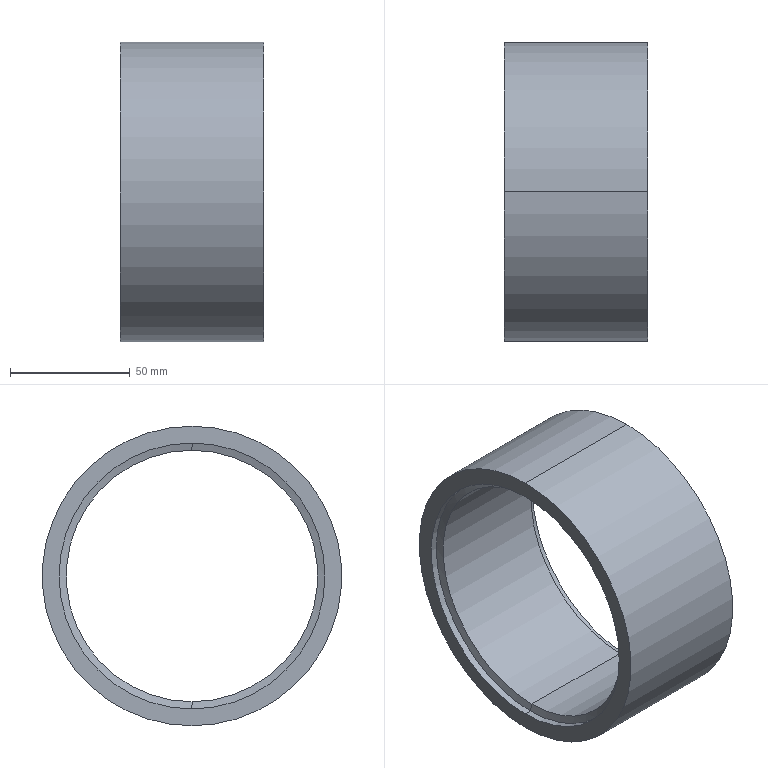Part | SolidWorks | features BaseBody 1 | 1 solid | 14 faces | box 60 x 125 x 125 mm | volume 209654 mm3 | cylinder 8 | cone 4 | plane 2 | commonest cylinder face diameters 111 x4 105 x2 125 x2
STEP:
#1=CARTESIAN_POINT('',(-30.,0.,-62.5));
#2=VERTEX_POINT('',#1);
#3=CARTESIAN_POINT('',(-30.,0.,62.5));
#4=VERTEX_POINT('',#3);
#5=CARTESIAN_POINT('',(-30.,0.,0.));
#6=DIRECTION('',(1.,0.,0.));
#7=DIRECTION('',(0.,0.,-1.));
#8=AXIS2_PLACEMENT_3D('',#5,#6,#7);
#9=CIRCLE('',#8,62.5);
#10=EDGE_CURVE('',#2,#4,#9,.T.);
#11=ORIENTED_EDGE('',*,*,#10,.T.);
#12=CARTESIAN_POINT('',(30.,0.,62.5));
#13=VERTEX_POINT('',#12);
#14=CARTESIAN_POINT('',(-33.,0.,62.5));
#15=DIRECTION('',(1.,0.,0.));
#16=VECTOR('',#15,1000.);
#17=LINE('',#14,#16);
#18=EDGE_CURVE('',#4,#13,#17,.T.);
#19=ORIENTED_EDGE('',*,*,#18,.T.);
#20=CARTESIAN_POINT('',(30.,0.,-62.5));
#21=VERTEX_POINT('',#20);
#22=CARTESIAN_POINT('',(30.,0.,0.));
#23=DIRECTION('',(-1.,0.,0.));
#24=DIRECTION('',(0.,0.,-1.));
#25=AXIS2_PLACEMENT_3D('',#22,#23,#24);
#26=CIRCLE('',#25,62.5);
#27=EDGE_CURVE('',#13,#21,#26,.T.);
#28=ORIENTED_EDGE('',*,*,#27,.T.);
#29=CARTESIAN_POINT('',(-33.,0.,-62.5));
#30=DIRECTION('',(1.,0.,0.));
#31=VECTOR('',#30,1000.);
#32=LINE('',#29,#31);
#33=EDGE_CURVE('',#2,#21,#32,.T.);
#34=ORIENTED_EDGE('',*,*,#33,.F.);
#35=EDGE_LOOP('',(#11,#19,#28,#34));
#36=FACE_OUTER_BOUND('',#35,.T.);
#37=CARTESIAN_POINT('',(-33.,0.,0.));
#38=DIRECTION('',(1.,0.,0.));
#39=DIRECTION('',(0.,0.,-1.));
#40=AXIS2_PLACEMENT_3D('',#37,#38,#39);
#41=CYLINDRICAL_SURFACE('',#40,62.5);
#42=ADVANCED_FACE('',(#36),#41,.T.);
#43=CARTESIAN_POINT('',(27.,0.,55.5));
#44=VERTEX_POINT('',#43);
#45=CARTESIAN_POINT('',(27.,0.,-55.5));
#46=VERTEX_POINT('',#45);
#47=CARTESIAN_POINT('',(27.,0.,0.));
#48=DIRECTION('',(1.,0.,0.));
#49=DIRECTION('',(0.,0.,-1.));
#50=AXIS2_PLACEMENT_3D('',#47,#48,#49);
#51=CIRCLE('',#50,55.5);
#52=EDGE_CURVE('',#44,#46,#51,.T.);
#53=ORIENTED_EDGE('',*,*,#52,.F.);
#54=CARTESIAN_POINT('',(30.,0.,55.5));
#55=VERTEX_POINT('',#54);
#56=CARTESIAN_POINT('',(-33.,0.,55.5));
#57=DIRECTION('',(1.,0.,0.));
#58=VECTOR('',#57,1000.);
#59=LINE('',#56,#58);
#60=EDGE_CURVE('',#44,#55,#59,.T.);
#61=ORIENTED_EDGE('',*,*,#60,.T.);
#62=CARTESIAN_POINT('',(30.,0.,-55.5));
#63=VERTEX_POINT('',#62);
#64=CARTESIAN_POINT('',(30.,0.,0.));
#65=DIRECTION('',(-1.,0.,0.));
#66=DIRECTION('',(0.,0.,-1.));
#67=AXIS2_PLACEMENT_3D('',#64,#65,#66);
#68=CIRCLE('',#67,55.5);
#69=EDGE_CURVE('',#63,#55,#68,.T.);
#70=ORIENTED_EDGE('',*,*,#69,.F.);
#71=CARTESIAN_POINT('',(-33.,0.,-55.5));
#72=DIRECTION('',(1.,0.,0.));
#73=VECTOR('',#72,1000.);
#74=LINE('',#71,#73);
#75=EDGE_CURVE('',#46,#63,#74,.T.);
#76=ORIENTED_EDGE('',*,*,#75,.F.);
#77=EDGE_LOOP('',(#53,#61,#70,#76));
#78=FACE_OUTER_BOUND('',#77,.T.);
#79=CARTESIAN_POINT('',(-33.,0.,0.));
#80=DIRECTION('',(1.,0.,0.));
#81=DIRECTION('',(0.,0.,-1.));
#82=AXIS2_PLACEMENT_3D('',#79,#80,#81);
#83=CYLINDRICAL_SURFACE('',#82,55.5);
#84=ADVANCED_FACE('',(#78),#83,.F.);
#85=CARTESIAN_POINT('',(-30.,0.,-55.5));
#86=VERTEX_POINT('',#85);
#87=CARTESIAN_POINT('',(-30.,0.,55.5));
#88=VERTEX_POINT('',#87);
#89=CARTESIAN_POINT('',(-30.,0.,0.));
#90=DIRECTION('',(-1.,0.,0.));
#91=DIRECTION('',(0.,0.,-1.));
#92=AXIS2_PLACEMENT_3D('',#89,#90,#91);
#93=CIRCLE('',#92,55.5);
#94=EDGE_CURVE('',#86,#88,#93,.T.);
#95=ORIENTED_EDGE('',*,*,#94,.T.);
#96=CARTESIAN_POINT('',(-27.,0.,55.5));
#97=VERTEX_POINT('',#96);
#98=CARTESIAN_POINT('',(-33.,0.,55.5));
#99=DIRECTION('',(1.,0.,0.));
#100=VECTOR('',#99,1000.);
#101=LINE('',#98,#100);
#102=EDGE_CURVE('',#88,#97,#101,.T.);
#103=ORIENTED_EDGE('',*,*,#102,.T.);
#104=CARTESIAN_POINT('',(-27.,0.,-55.5));
#105=VERTEX_POINT('',#104);
#106=CARTESIAN_POINT('',(-27.,0.,0.));
#107=DIRECTION('',(-1.,0.,0.));
#108=DIRECTION('',(0.,0.,-1.));
#109=AXIS2_PLACEMENT_3D('',#106,#107,#108);
#110=CIRCLE('',#109,55.5);
#111=EDGE_CURVE('',#105,#97,#110,.T.);
#112=ORIENTED_EDGE('',*,*,#111,.F.);
#113=CARTESIAN_POINT('',(-33.,0.,-55.5));
#114=DIRECTION('',(1.,0.,0.));
#115=VECTOR('',#114,1000.);
#116=LINE('',#113,#115);
#117=EDGE_CURVE('',#86,#105,#116,.T.);
#118=ORIENTED_EDGE('',*,*,#117,.F.);
#119=EDGE_LOOP('',(#95,#103,#112,#118));
#120=FACE_OUTER_BOUND('',#119,.T.);
#121=CARTESIAN_POINT('',(-33.,0.,0.));
#122=DIRECTION('',(1.,0.,0.));
#123=DIRECTION('',(0.,0.,-1.));
#124=AXIS2_PLACEMENT_3D('',#121,#122,#123);
#125=CYLINDRICAL_SURFACE('',#124,55.5);
#126=ADVANCED_FACE('',(#120),#125,.F.);
#127=CARTESIAN_POINT('',(26.,0.,52.5));
#128=VERTEX_POINT('',#127);
#129=CARTESIAN_POINT('',(26.,0.,-52.5));
#130=VERTEX_POINT('',#129);
#131=CARTESIAN_POINT('',(26.,0.,0.));
#132=DIRECTION('',(1.,0.,0.));
#133=DIRECTION('',(0.,0.,1.));
#134=AXIS2_PLACEMENT_3D('',#131,#132,#133);
#135=CIRCLE('',#134,52.5);
#136=EDGE_CURVE('',#128,#130,#135,.T.);
#137=ORIENTED_EDGE('',*,*,#136,.F.);
#138=CARTESIAN_POINT('',(27.,0.,55.5));
#139=DIRECTION('',(0.3162,0.,0.9487));
#140=VECTOR('',#139,1000.);
#141=LINE('',#138,#140);
#142=EDGE_CURVE('',#128,#44,#141,.T.);
#143=ORIENTED_EDGE('',*,*,#142,.T.);
#144=ORIENTED_EDGE('',*,*,#52,.T.);
#145=CARTESIAN_POINT('',(27.,0.,-55.5));
#146=DIRECTION('',(0.3162,0.,-0.9487));
#147=VECTOR('',#146,1000.);
#148=LINE('',#145,#147);
#149=EDGE_CURVE('',#130,#46,#148,.T.);
#150=ORIENTED_EDGE('',*,*,#149,.F.);
#151=EDGE_LOOP('',(#137,#143,#144,#150));
#152=FACE_OUTER_BOUND('',#151,.T.);
#153=CARTESIAN_POINT('',(27.,0.,0.));
#154=DIRECTION('',(1.,0.,0.));
#155=DIRECTION('',(0.,0.,-1.));
#156=AXIS2_PLACEMENT_3D('',#153,#154,#155);
#157=CONICAL_SURFACE('',#156,55.5,1.249);
#158=ADVANCED_FACE('',(#152),#157,.F.);
#159=CARTESIAN_POINT('',(-26.,0.,-52.5));
#160=VERTEX_POINT('',#159);
#161=CARTESIAN_POINT('',(-26.,0.,52.5));
#162=VERTEX_POINT('',#161);
#163=CARTESIAN_POINT('',(-26.,0.,0.));
#164=DIRECTION('',(-1.,0.,0.));
#165=DIRECTION('',(0.,0.,-1.));
#166=AXIS2_PLACEMENT_3D('',#163,#164,#165);
#167=CIRCLE('',#166,52.5);
#168=EDGE_CURVE('',#160,#162,#167,.T.);
#169=ORIENTED_EDGE('',*,*,#168,.F.);
#170=CARTESIAN_POINT('',(-27.,0.,-55.5));
#171=DIRECTION('',(-0.3162,0.,-0.9487));
#172=VECTOR('',#171,1000.);
#173=LINE('',#170,#172);
#174=EDGE_CURVE('',#160,#105,#173,.T.);
#175=ORIENTED_EDGE('',*,*,#174,.T.);
#176=ORIENTED_EDGE('',*,*,#111,.T.);
#177=CARTESIAN_POINT('',(-27.,0.,55.5));
#178=DIRECTION('',(-0.3162,0.,0.9487));
#179=VECTOR('',#178,1000.);
#180=LINE('',#177,#179);
#181=EDGE_CURVE('',#162,#97,#180,.T.);
#182=ORIENTED_EDGE('',*,*,#181,.F.);
#183=EDGE_LOOP('',(#169,#175,#176,#182));
#184=FACE_OUTER_BOUND('',#183,.T.);
#185=CARTESIAN_POINT('',(-27.,0.,0.));
#186=DIRECTION('',(-1.,0.,0.));
#187=DIRECTION('',(0.,0.,1.));
#188=AXIS2_PLACEMENT_3D('',#185,#186,#187);
#189=CONICAL_SURFACE('',#188,55.5,1.249);
#190=ADVANCED_FACE('',(#184),#189,.F.);
#191=ORIENTED_EDGE('',*,*,#168,.T.);
#192=CARTESIAN_POINT('',(-33.,0.,52.5));
#193=DIRECTION('',(1.,0.,0.));
#194=VECTOR('',#193,1000.);
#195=LINE('',#192,#194);
#196=EDGE_CURVE('',#162,#128,#195,.T.);
#197=ORIENTED_EDGE('',*,*,#196,.T.);
#198=ORIENTED_EDGE('',*,*,#136,.T.);
#199=CARTESIAN_POINT('',(-33.,0.,-52.5));
#200=DIRECTION('',(1.,0.,0.));
#201=VECTOR('',#200,1000.);
#202=LINE('',#199,#201);
#203=EDGE_CURVE('',#160,#130,#202,.T.);
#204=ORIENTED_EDGE('',*,*,#203,.F.);
#205=EDGE_LOOP('',(#191,#197,#198,#204));
#206=FACE_OUTER_BOUND('',#205,.T.);
#207=CARTESIAN_POINT('',(-33.,0.,0.));
#208=DIRECTION('',(1.,0.,0.));
#209=DIRECTION('',(0.,0.,-1.));
#210=AXIS2_PLACEMENT_3D('',#207,#208,#209);
#211=CYLINDRICAL_SURFACE('',#210,52.5);
#212=ADVANCED_FACE('',(#206),#211,.F.);
#213=ORIENTED_EDGE('',*,*,#18,.F.);
#214=CARTESIAN_POINT('',(-30.,0.,0.));
#215=DIRECTION('',(1.,0.,0.));
#216=DIRECTION('',(0.,0.,-1.));
#217=AXIS2_PLACEMENT_3D('',#214,#215,#216);
#218=CIRCLE('',#217,62.5);
#219=EDGE_CURVE('',#4,#2,#218,.T.);
#220=ORIENTED_EDGE('',*,*,#219,.T.);
#221=ORIENTED_EDGE('',*,*,#33,.T.);
#222=CARTESIAN_POINT('',(30.,0.,0.));
#223=DIRECTION('',(-1.,0.,0.));
#224=DIRECTION('',(0.,0.,-1.));
#225=AXIS2_PLACEMENT_3D('',#222,#223,#224);
#226=CIRCLE('',#225,62.5);
#227=EDGE_CURVE('',#21,#13,#226,.T.);
#228=ORIENTED_EDGE('',*,*,#227,.T.);
#229=EDGE_LOOP('',(#213,#220,#221,#228));
#230=FACE_OUTER_BOUND('',#229,.T.);
#231=CARTESIAN_POINT('',(-33.,0.,0.));
#232=DIRECTION('',(1.,0.,0.));
#233=DIRECTION('',(0.,0.,-1.));
#234=AXIS2_PLACEMENT_3D('',#231,#232,#233);
#235=CYLINDRICAL_SURFACE('',#234,62.5);
#236=ADVANCED_FACE('',(#230),#235,.T.);
#237=ORIENTED_EDGE('',*,*,#69,.T.);
#238=CARTESIAN_POINT('',(30.,0.,0.));
#239=DIRECTION('',(-1.,0.,0.));
#240=DIRECTION('',(0.,0.,-1.));
#241=AXIS2_PLACEMENT_3D('',#238,#239,#240);
#242=CIRCLE('',#241,55.5);
#243=EDGE_CURVE('',#55,#63,#242,.T.);
#244=ORIENTED_EDGE('',*,*,#243,.T.);
#245=EDGE_LOOP('',(#237,#244));
#246=FACE_BOUND('',#245,.T.);
#247=ORIENTED_EDGE('',*,*,#227,.F.);
#248=ORIENTED_EDGE('',*,*,#27,.F.);
#249=EDGE_LOOP('',(#247,#248));
#250=FACE_OUTER_BOUND('',#249,.T.);
#251=CARTESIAN_POINT('',(30.,0.,0.));
#252=DIRECTION('',(1.,0.,0.));
#253=DIRECTION('',(0.,0.,-1.));
#254=AXIS2_PLACEMENT_3D('',#251,#252,#253);
#255=PLANE('',#254);
#256=ADVANCED_FACE('',(#246,#250),#255,.T.);
#257=ORIENTED_EDGE('',*,*,#94,.F.);
#258=CARTESIAN_POINT('',(-30.,0.,0.));
#259=DIRECTION('',(-1.,0.,0.));
#260=DIRECTION('',(0.,0.,-1.));
#261=AXIS2_PLACEMENT_3D('',#258,#259,#260);
#262=CIRCLE('',#261,55.5);
#263=EDGE_CURVE('',#88,#86,#262,.T.);
#264=ORIENTED_EDGE('',*,*,#263,.F.);
#265=EDGE_LOOP('',(#257,#264));
#266=FACE_BOUND('',#265,.T.);
#267=ORIENTED_EDGE('',*,*,#10,.F.);
#268=ORIENTED_EDGE('',*,*,#219,.F.);
#269=EDGE_LOOP('',(#267,#268));
#270=FACE_OUTER_BOUND('',#269,.T.);
#271=CARTESIAN_POINT('',(-30.,0.,0.));
#272=DIRECTION('',(1.,0.,0.));
#273=DIRECTION('',(0.,0.,-1.));
#274=AXIS2_PLACEMENT_3D('',#271,#272,#273);
#275=PLANE('',#274);
#276=ADVANCED_FACE('',(#266,#270),#275,.F.);
#277=ORIENTED_EDGE('',*,*,#60,.F.);
#278=CARTESIAN_POINT('',(27.,0.,0.));
#279=DIRECTION('',(1.,0.,0.));
#280=DIRECTION('',(0.,0.,-1.));
#281=AXIS2_PLACEMENT_3D('',#278,#279,#280);
#282=CIRCLE('',#281,55.5);
#283=EDGE_CURVE('',#46,#44,#282,.T.);
#284=ORIENTED_EDGE('',*,*,#283,.F.);
#285=ORIENTED_EDGE('',*,*,#75,.T.);
#286=ORIENTED_EDGE('',*,*,#243,.F.);
#287=EDGE_LOOP('',(#277,#284,#285,#286));
#288=FACE_OUTER_BOUND('',#287,.T.);
#289=CARTESIAN_POINT('',(-33.,0.,0.));
#290=DIRECTION('',(1.,0.,0.));
#291=DIRECTION('',(0.,0.,-1.));
#292=AXIS2_PLACEMENT_3D('',#289,#290,#291);
#293=CYLINDRICAL_SURFACE('',#292,55.5);
#294=ADVANCED_FACE('',(#288),#293,.F.);
#295=ORIENTED_EDGE('',*,*,#102,.F.);
#296=ORIENTED_EDGE('',*,*,#263,.T.);
#297=ORIENTED_EDGE('',*,*,#117,.T.);
#298=CARTESIAN_POINT('',(-27.,0.,0.));
#299=DIRECTION('',(-1.,0.,0.));
#300=DIRECTION('',(0.,0.,-1.));
#301=AXIS2_PLACEMENT_3D('',#298,#299,#300);
#302=CIRCLE('',#301,55.5);
#303=EDGE_CURVE('',#97,#105,#302,.T.);
#304=ORIENTED_EDGE('',*,*,#303,.F.);
#305=EDGE_LOOP('',(#295,#296,#297,#304));
#306=FACE_OUTER_BOUND('',#305,.T.);
#307=CARTESIAN_POINT('',(-33.,0.,0.));
#308=DIRECTION('',(1.,0.,0.));
#309=DIRECTION('',(0.,0.,-1.));
#310=AXIS2_PLACEMENT_3D('',#307,#308,#309);
#311=CYLINDRICAL_SURFACE('',#310,55.5);
#312=ADVANCED_FACE('',(#306),#311,.F.);
#313=ORIENTED_EDGE('',*,*,#142,.F.);
#314=CARTESIAN_POINT('',(26.,0.,0.));
#315=DIRECTION('',(1.,0.,0.));
#316=DIRECTION('',(0.,0.,1.));
#317=AXIS2_PLACEMENT_3D('',#314,#315,#316);
#318=CIRCLE('',#317,52.5);
#319=EDGE_CURVE('',#130,#128,#318,.T.);
#320=ORIENTED_EDGE('',*,*,#319,.F.);
#321=ORIENTED_EDGE('',*,*,#149,.T.);
#322=ORIENTED_EDGE('',*,*,#283,.T.);
#323=EDGE_LOOP('',(#313,#320,#321,#322));
#324=FACE_OUTER_BOUND('',#323,.T.);
#325=CARTESIAN_POINT('',(27.,0.,0.));
#326=DIRECTION('',(1.,0.,0.));
#327=DIRECTION('',(0.,0.,-1.));
#328=AXIS2_PLACEMENT_3D('',#325,#326,#327);
#329=CONICAL_SURFACE('',#328,55.5,1.249);
#330=ADVANCED_FACE('',(#324),#329,.F.);
#331=ORIENTED_EDGE('',*,*,#174,.F.);
#332=CARTESIAN_POINT('',(-26.,0.,0.));
#333=DIRECTION('',(-1.,0.,0.));
#334=DIRECTION('',(0.,0.,-1.));
#335=AXIS2_PLACEMENT_3D('',#332,#333,#334);
#336=CIRCLE('',#335,52.5);
#337=EDGE_CURVE('',#162,#160,#336,.T.);
#338=ORIENTED_EDGE('',*,*,#337,.F.);
#339=ORIENTED_EDGE('',*,*,#181,.T.);
#340=ORIENTED_EDGE('',*,*,#303,.T.);
#341=EDGE_LOOP('',(#331,#338,#339,#340));
#342=FACE_OUTER_BOUND('',#341,.T.);
#343=CARTESIAN_POINT('',(-27.,0.,0.));
#344=DIRECTION('',(-1.,0.,0.));
#345=DIRECTION('',(0.,0.,1.));
#346=AXIS2_PLACEMENT_3D('',#343,#344,#345);
#347=CONICAL_SURFACE('',#346,55.5,1.249);
#348=ADVANCED_FACE('',(#342),#347,.F.);
#349=ORIENTED_EDGE('',*,*,#196,.F.);
#350=ORIENTED_EDGE('',*,*,#337,.T.);
#351=ORIENTED_EDGE('',*,*,#203,.T.);
#352=ORIENTED_EDGE('',*,*,#319,.T.);
#353=EDGE_LOOP('',(#349,#350,#351,#352));
#354=FACE_OUTER_BOUND('',#353,.T.);
#355=CARTESIAN_POINT('',(-33.,0.,0.));
#356=DIRECTION('',(1.,0.,0.));
#357=DIRECTION('',(0.,0.,-1.));
#358=AXIS2_PLACEMENT_3D('',#355,#356,#357);
#359=CYLINDRICAL_SURFACE('',#358,52.5);
#360=ADVANCED_FACE('',(#354),#359,.F.);
#361=CLOSED_SHELL('',(#42,#84,#126,#158,#190,#212,#236,#256,#276,#294,#312,#330,#348,#360));
#362=MANIFOLD_SOLID_BREP('',#361);
#363=CARTESIAN_POINT('',(0.,0.,0.));
#364=DIRECTION('',(0.,0.,1.));
#365=DIRECTION('',(1.,0.,0.));
#366=AXIS2_PLACEMENT_3D('',#363,#364,#365);
#367=(LENGTH_UNIT()NAMED_UNIT(*)SI_UNIT(.MILLI.,.METRE.));
#368=UNCERTAINTY_MEASURE_WITH_UNIT(LENGTH_MEASURE(0.00001),#367,'','');
#369=(NAMED_UNIT(*)PLANE_ANGLE_UNIT()SI_UNIT($,.RADIAN.));
#370=(NAMED_UNIT(*)SI_UNIT($,.STERADIAN.)SOLID_ANGLE_UNIT());
#371=(GEOMETRIC_REPRESENTATION_CONTEXT(3)GLOBAL_UNCERTAINTY_ASSIGNED_CONTEXT((#368))GLOBAL_UNIT_ASSIGNED_CONTEXT((#367,#369,#370))REPRESENTATION_CONTEXT('',''));
#372=ADVANCED_BREP_SHAPE_REPRESENTATION('',(#362,#366),#371);